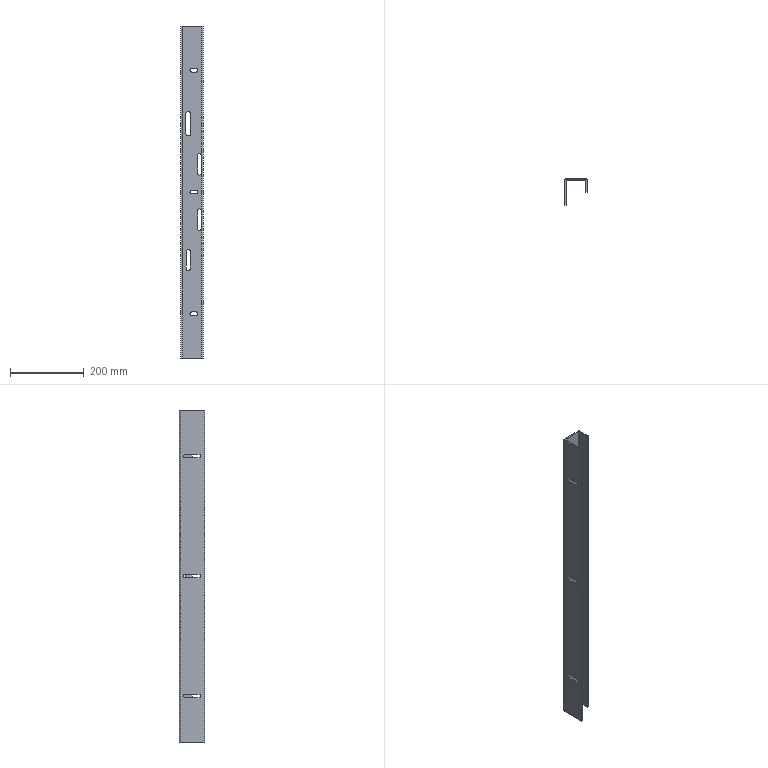Part | 1 solid | 71 faces | box 60 x 70 x 900 mm | volume 411607 mm3 | plane 38 | cylinder 33 | commonest cylinder face diameters 10 x21 7 x6 0.4 x2 6.4 x2 14 x2